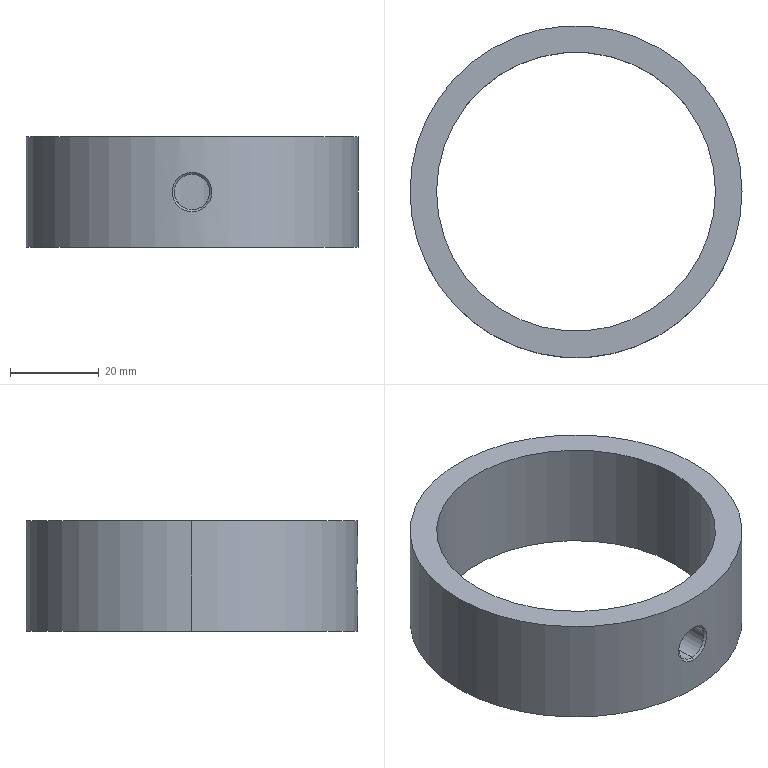Part | SolidWorks | features Chamfer 1, Extrusion 1, ICE 1 | 1 solid | 10 faces | box 75 x 75 x 25 mm | volume 32210 mm3 | cylinder 6 | spline 2 | plane 2 | commonest cylinder face diameters 8 x2 63 x2 75 x2